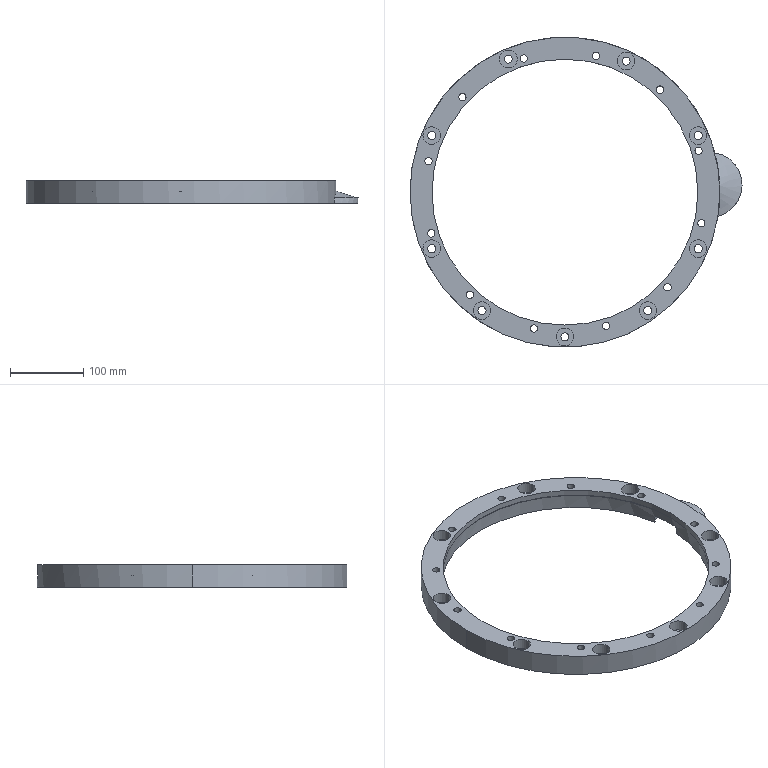Part | SolidWorks | features BaseBody 1 | 1 solid | 86 faces | box 452.148 x 422 x 30.2 mm | volume 967306 mm3 | cylinder 69 | plane 12 | spline 5 | commonest cylinder face diameters 10 x24 11 x18 24 x18 50 x2 362 x2 366 x2